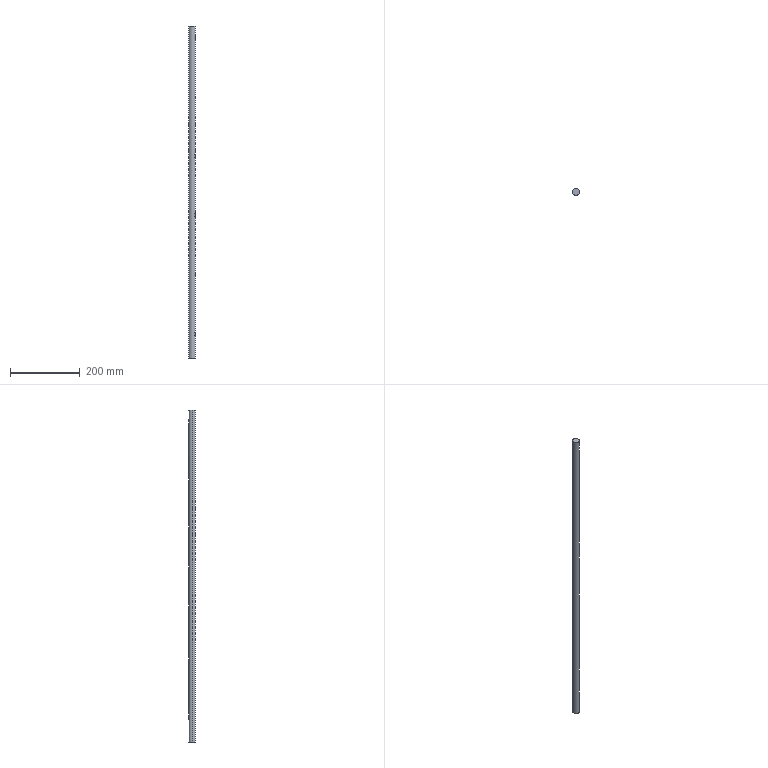Part | SolidWorks | features BaseBody 1 | 1 solid | 40 faces | box 20 x 20 x 952 mm | volume 298375 mm3 | plane 38 | cylinder 2 | commonest cylinder face diameters 20 x2
STEP:
#1=CARTESIAN_POINT('',(4.359,9.,914.5));
#2=VERTEX_POINT('',#1);
#3=CARTESIAN_POINT('',(-4.359,9.,914.5));
#4=VERTEX_POINT('',#3);
#5=CARTESIAN_POINT('',(0.,0.,914.5));
#6=DIRECTION('',(0.,0.,1.));
#7=DIRECTION('',(1.,0.,0.));
#8=AXIS2_PLACEMENT_3D('',#5,#6,#7);
#9=CIRCLE('',#8,10.);
#10=EDGE_CURVE('',#2,#4,#9,.T.);
#11=ORIENTED_EDGE('',*,*,#10,.F.);
#12=CARTESIAN_POINT('',(4.359,9.,924.5));
#13=VERTEX_POINT('',#12);
#14=CARTESIAN_POINT('',(4.359,9.,952.));
#15=DIRECTION('',(0.,0.,1.));
#16=VECTOR('',#15,1000.);
#17=LINE('',#14,#16);
#18=EDGE_CURVE('',#2,#13,#17,.T.);
#19=ORIENTED_EDGE('',*,*,#18,.T.);
#20=CARTESIAN_POINT('',(-4.359,9.,924.5));
#21=VERTEX_POINT('',#20);
#22=CARTESIAN_POINT('',(0.,0.,924.5));
#23=DIRECTION('',(0.,0.,1.));
#24=DIRECTION('',(1.,0.,0.));
#25=AXIS2_PLACEMENT_3D('',#22,#23,#24);
#26=CIRCLE('',#25,10.);
#27=EDGE_CURVE('',#13,#21,#26,.T.);
#28=ORIENTED_EDGE('',*,*,#27,.T.);
#29=CARTESIAN_POINT('',(-4.359,9.,952.));
#30=DIRECTION('',(0.,0.,-1.));
#31=VECTOR('',#30,1000.);
#32=LINE('',#29,#31);
#33=EDGE_CURVE('',#21,#4,#32,.T.);
#34=ORIENTED_EDGE('',*,*,#33,.T.);
#35=EDGE_LOOP('',(#11,#19,#28,#34));
#36=FACE_BOUND('',#35,.T.);
#37=CARTESIAN_POINT('',(4.359,9.,744.5));
#38=VERTEX_POINT('',#37);
#39=CARTESIAN_POINT('',(-4.359,9.,744.5));
#40=VERTEX_POINT('',#39);
#41=CARTESIAN_POINT('',(0.,0.,744.5));
#42=DIRECTION('',(0.,0.,1.));
#43=DIRECTION('',(1.,0.,0.));
#44=AXIS2_PLACEMENT_3D('',#41,#42,#43);
#45=CIRCLE('',#44,10.);
#46=EDGE_CURVE('',#38,#40,#45,.T.);
#47=ORIENTED_EDGE('',*,*,#46,.F.);
#48=CARTESIAN_POINT('',(4.359,9.,754.5));
#49=VERTEX_POINT('',#48);
#50=CARTESIAN_POINT('',(4.359,9.,952.));
#51=DIRECTION('',(0.,0.,1.));
#52=VECTOR('',#51,1000.);
#53=LINE('',#50,#52);
#54=EDGE_CURVE('',#38,#49,#53,.T.);
#55=ORIENTED_EDGE('',*,*,#54,.T.);
#56=CARTESIAN_POINT('',(-4.359,9.,754.5));
#57=VERTEX_POINT('',#56);
#58=CARTESIAN_POINT('',(0.,0.,754.5));
#59=DIRECTION('',(0.,0.,1.));
#60=DIRECTION('',(1.,0.,0.));
#61=AXIS2_PLACEMENT_3D('',#58,#59,#60);
#62=CIRCLE('',#61,10.);
#63=EDGE_CURVE('',#49,#57,#62,.T.);
#64=ORIENTED_EDGE('',*,*,#63,.T.);
#65=CARTESIAN_POINT('',(-4.359,9.,952.));
#66=DIRECTION('',(0.,0.,-1.));
#67=VECTOR('',#66,1000.);
#68=LINE('',#65,#67);
#69=EDGE_CURVE('',#57,#40,#68,.T.);
#70=ORIENTED_EDGE('',*,*,#69,.T.);
#71=EDGE_LOOP('',(#47,#55,#64,#70));
#72=FACE_BOUND('',#71,.T.);
#73=CARTESIAN_POINT('',(4.359,9.,574.5));
#74=VERTEX_POINT('',#73);
#75=CARTESIAN_POINT('',(-4.359,9.,574.5));
#76=VERTEX_POINT('',#75);
#77=CARTESIAN_POINT('',(0.,0.,574.5));
#78=DIRECTION('',(0.,0.,1.));
#79=DIRECTION('',(1.,0.,0.));
#80=AXIS2_PLACEMENT_3D('',#77,#78,#79);
#81=CIRCLE('',#80,10.);
#82=EDGE_CURVE('',#74,#76,#81,.T.);
#83=ORIENTED_EDGE('',*,*,#82,.F.);
#84=CARTESIAN_POINT('',(4.359,9.,584.5));
#85=VERTEX_POINT('',#84);
#86=CARTESIAN_POINT('',(4.359,9.,952.));
#87=DIRECTION('',(0.,0.,1.));
#88=VECTOR('',#87,1000.);
#89=LINE('',#86,#88);
#90=EDGE_CURVE('',#74,#85,#89,.T.);
#91=ORIENTED_EDGE('',*,*,#90,.T.);
#92=CARTESIAN_POINT('',(-4.359,9.,584.5));
#93=VERTEX_POINT('',#92);
#94=CARTESIAN_POINT('',(0.,0.,584.5));
#95=DIRECTION('',(0.,0.,1.));
#96=DIRECTION('',(1.,0.,0.));
#97=AXIS2_PLACEMENT_3D('',#94,#95,#96);
#98=CIRCLE('',#97,10.);
#99=EDGE_CURVE('',#85,#93,#98,.T.);
#100=ORIENTED_EDGE('',*,*,#99,.T.);
#101=CARTESIAN_POINT('',(-4.359,9.,952.));
#102=DIRECTION('',(0.,0.,-1.));
#103=VECTOR('',#102,1000.);
#104=LINE('',#101,#103);
#105=EDGE_CURVE('',#93,#76,#104,.T.);
#106=ORIENTED_EDGE('',*,*,#105,.T.);
#107=EDGE_LOOP('',(#83,#91,#100,#106));
#108=FACE_BOUND('',#107,.T.);
#109=CARTESIAN_POINT('',(4.359,9.,404.5));
#110=VERTEX_POINT('',#109);
#111=CARTESIAN_POINT('',(-4.359,9.,404.5));
#112=VERTEX_POINT('',#111);
#113=CARTESIAN_POINT('',(0.,0.,404.5));
#114=DIRECTION('',(0.,0.,1.));
#115=DIRECTION('',(1.,0.,0.));
#116=AXIS2_PLACEMENT_3D('',#113,#114,#115);
#117=CIRCLE('',#116,10.);
#118=EDGE_CURVE('',#110,#112,#117,.T.);
#119=ORIENTED_EDGE('',*,*,#118,.F.);
#120=CARTESIAN_POINT('',(4.359,9.,414.5));
#121=VERTEX_POINT('',#120);
#122=CARTESIAN_POINT('',(4.359,9.,952.));
#123=DIRECTION('',(0.,0.,1.));
#124=VECTOR('',#123,1000.);
#125=LINE('',#122,#124);
#126=EDGE_CURVE('',#110,#121,#125,.T.);
#127=ORIENTED_EDGE('',*,*,#126,.T.);
#128=CARTESIAN_POINT('',(-4.359,9.,414.5));
#129=VERTEX_POINT('',#128);
#130=CARTESIAN_POINT('',(0.,0.,414.5));
#131=DIRECTION('',(0.,0.,1.));
#132=DIRECTION('',(1.,0.,0.));
#133=AXIS2_PLACEMENT_3D('',#130,#131,#132);
#134=CIRCLE('',#133,10.);
#135=EDGE_CURVE('',#121,#129,#134,.T.);
#136=ORIENTED_EDGE('',*,*,#135,.T.);
#137=CARTESIAN_POINT('',(-4.359,9.,952.));
#138=DIRECTION('',(0.,0.,-1.));
#139=VECTOR('',#138,1000.);
#140=LINE('',#137,#139);
#141=EDGE_CURVE('',#129,#112,#140,.T.);
#142=ORIENTED_EDGE('',*,*,#141,.T.);
#143=EDGE_LOOP('',(#119,#127,#136,#142));
#144=FACE_BOUND('',#143,.T.);
#145=CARTESIAN_POINT('',(4.359,9.,234.5));
#146=VERTEX_POINT('',#145);
#147=CARTESIAN_POINT('',(-4.359,9.,234.5));
#148=VERTEX_POINT('',#147);
#149=CARTESIAN_POINT('',(0.,0.,234.5));
#150=DIRECTION('',(0.,0.,1.));
#151=DIRECTION('',(1.,0.,0.));
#152=AXIS2_PLACEMENT_3D('',#149,#150,#151);
#153=CIRCLE('',#152,10.);
#154=EDGE_CURVE('',#146,#148,#153,.T.);
#155=ORIENTED_EDGE('',*,*,#154,.F.);
#156=CARTESIAN_POINT('',(4.359,9.,244.5));
#157=VERTEX_POINT('',#156);
#158=CARTESIAN_POINT('',(4.359,9.,952.));
#159=DIRECTION('',(0.,0.,1.));
#160=VECTOR('',#159,1000.);
#161=LINE('',#158,#160);
#162=EDGE_CURVE('',#146,#157,#161,.T.);
#163=ORIENTED_EDGE('',*,*,#162,.T.);
#164=CARTESIAN_POINT('',(-4.359,9.,244.5));
#165=VERTEX_POINT('',#164);
#166=CARTESIAN_POINT('',(0.,0.,244.5));
#167=DIRECTION('',(0.,0.,1.));
#168=DIRECTION('',(1.,0.,0.));
#169=AXIS2_PLACEMENT_3D('',#166,#167,#168);
#170=CIRCLE('',#169,10.);
#171=EDGE_CURVE('',#157,#165,#170,.T.);
#172=ORIENTED_EDGE('',*,*,#171,.T.);
#173=CARTESIAN_POINT('',(-4.359,9.,952.));
#174=DIRECTION('',(0.,0.,-1.));
#175=VECTOR('',#174,1000.);
#176=LINE('',#173,#175);
#177=EDGE_CURVE('',#165,#148,#176,.T.);
#178=ORIENTED_EDGE('',*,*,#177,.T.);
#179=EDGE_LOOP('',(#155,#163,#172,#178));
#180=FACE_BOUND('',#179,.T.);
#181=CARTESIAN_POINT('',(4.359,9.,64.5));
#182=VERTEX_POINT('',#181);
#183=CARTESIAN_POINT('',(-4.359,9.,64.5));
#184=VERTEX_POINT('',#183);
#185=CARTESIAN_POINT('',(0.,0.,64.5));
#186=DIRECTION('',(0.,0.,1.));
#187=DIRECTION('',(1.,0.,0.));
#188=AXIS2_PLACEMENT_3D('',#185,#186,#187);
#189=CIRCLE('',#188,10.);
#190=EDGE_CURVE('',#182,#184,#189,.T.);
#191=ORIENTED_EDGE('',*,*,#190,.F.);
#192=CARTESIAN_POINT('',(4.359,9.,74.5));
#193=VERTEX_POINT('',#192);
#194=CARTESIAN_POINT('',(4.359,9.,952.));
#195=DIRECTION('',(0.,0.,1.));
#196=VECTOR('',#195,1000.);
#197=LINE('',#194,#196);
#198=EDGE_CURVE('',#182,#193,#197,.T.);
#199=ORIENTED_EDGE('',*,*,#198,.T.);
#200=CARTESIAN_POINT('',(-4.359,9.,74.5));
#201=VERTEX_POINT('',#200);
#202=CARTESIAN_POINT('',(0.,0.,74.5));
#203=DIRECTION('',(0.,0.,1.));
#204=DIRECTION('',(1.,0.,0.));
#205=AXIS2_PLACEMENT_3D('',#202,#203,#204);
#206=CIRCLE('',#205,10.);
#207=EDGE_CURVE('',#193,#201,#206,.T.);
#208=ORIENTED_EDGE('',*,*,#207,.T.);
#209=CARTESIAN_POINT('',(-4.359,9.,952.));
#210=DIRECTION('',(0.,0.,-1.));
#211=VECTOR('',#210,1000.);
#212=LINE('',#209,#211);
#213=EDGE_CURVE('',#201,#184,#212,.T.);
#214=ORIENTED_EDGE('',*,*,#213,.T.);
#215=EDGE_LOOP('',(#191,#199,#208,#214));
#216=FACE_BOUND('',#215,.T.);
#217=CARTESIAN_POINT('',(10.,0.,952.));
#218=VERTEX_POINT('',#217);
#219=CARTESIAN_POINT('',(-10.,0.,952.));
#220=VERTEX_POINT('',#219);
#221=CARTESIAN_POINT('',(0.,0.,952.));
#222=DIRECTION('',(0.,0.,1.));
#223=DIRECTION('',(1.,0.,0.));
#224=AXIS2_PLACEMENT_3D('',#221,#222,#223);
#225=CIRCLE('',#224,10.);
#226=EDGE_CURVE('',#218,#220,#225,.T.);
#227=ORIENTED_EDGE('',*,*,#226,.F.);
#228=CARTESIAN_POINT('',(10.,0.,0.));
#229=VERTEX_POINT('',#228);
#230=CARTESIAN_POINT('',(10.,0.,952.));
#231=DIRECTION('',(0.,0.,-1.));
#232=VECTOR('',#231,1000.);
#233=LINE('',#230,#232);
#234=EDGE_CURVE('',#218,#229,#233,.T.);
#235=ORIENTED_EDGE('',*,*,#234,.T.);
#236=CARTESIAN_POINT('',(-10.,0.,0.));
#237=VERTEX_POINT('',#236);
#238=CARTESIAN_POINT('',(0.,0.,0.));
#239=DIRECTION('',(0.,0.,1.));
#240=DIRECTION('',(1.,0.,0.));
#241=AXIS2_PLACEMENT_3D('',#238,#239,#240);
#242=CIRCLE('',#241,10.);
#243=EDGE_CURVE('',#229,#237,#242,.T.);
#244=ORIENTED_EDGE('',*,*,#243,.T.);
#245=CARTESIAN_POINT('',(-10.,0.,952.));
#246=DIRECTION('',(0.,0.,-1.));
#247=VECTOR('',#246,1000.);
#248=LINE('',#245,#247);
#249=EDGE_CURVE('',#220,#237,#248,.T.);
#250=ORIENTED_EDGE('',*,*,#249,.F.);
#251=EDGE_LOOP('',(#227,#235,#244,#250));
#252=FACE_OUTER_BOUND('',#251,.T.);
#253=CARTESIAN_POINT('',(0.,0.,952.));
#254=DIRECTION('',(0.,0.,-1.));
#255=DIRECTION('',(-1.,0.,0.));
#256=AXIS2_PLACEMENT_3D('',#253,#254,#255);
#257=CYLINDRICAL_SURFACE('',#256,10.);
#258=ADVANCED_FACE('',(#36,#72,#108,#144,#180,#216,#252),#257,.T.);
#259=CARTESIAN_POINT('',(9.974,-0.7251,74.5));
#260=VERTEX_POINT('',#259);
#261=CARTESIAN_POINT('',(5.615,-8.275,74.5));
#262=VERTEX_POINT('',#261);
#263=CARTESIAN_POINT('',(12.917,4.373,74.5));
#264=DIRECTION('',(-0.5,-0.866,0.));
#265=VECTOR('',#264,1000.);
#266=LINE('',#263,#265);
#267=EDGE_CURVE('',#260,#262,#266,.T.);
#268=ORIENTED_EDGE('',*,*,#267,.F.);
#269=CARTESIAN_POINT('',(0.,0.,74.5));
#270=DIRECTION('',(0.,0.,1.));
#271=DIRECTION('',(1.,0.,0.));
#272=AXIS2_PLACEMENT_3D('',#269,#270,#271);
#273=CIRCLE('',#272,10.);
#274=EDGE_CURVE('',#262,#260,#273,.T.);
#275=ORIENTED_EDGE('',*,*,#274,.F.);
#276=EDGE_LOOP('',(#268,#275));
#277=FACE_OUTER_BOUND('',#276,.T.);
#278=CARTESIAN_POINT('',(0.,0.,74.5));
#279=DIRECTION('',(0.,0.,1.));
#280=DIRECTION('',(1.,0.,0.));
#281=AXIS2_PLACEMENT_3D('',#278,#279,#280);
#282=PLANE('',#281);
#283=ADVANCED_FACE('',(#277),#282,.F.);
#284=CARTESIAN_POINT('',(5.615,-8.275,64.5));
#285=VERTEX_POINT('',#284);
#286=CARTESIAN_POINT('',(9.974,-0.7251,64.5));
#287=VERTEX_POINT('',#286);
#288=CARTESIAN_POINT('',(0.,0.,64.5));
#289=DIRECTION('',(0.,0.,1.));
#290=DIRECTION('',(1.,0.,0.));
#291=AXIS2_PLACEMENT_3D('',#288,#289,#290);
#292=CIRCLE('',#291,10.);
#293=EDGE_CURVE('',#285,#287,#292,.T.);
#294=ORIENTED_EDGE('',*,*,#293,.T.);
#295=CARTESIAN_POINT('',(12.917,4.373,64.5));
#296=DIRECTION('',(-0.5,-0.866,0.));
#297=VECTOR('',#296,1000.);
#298=LINE('',#295,#297);
#299=EDGE_CURVE('',#287,#285,#298,.T.);
#300=ORIENTED_EDGE('',*,*,#299,.T.);
#301=EDGE_LOOP('',(#294,#300));
#302=FACE_OUTER_BOUND('',#301,.T.);
#303=CARTESIAN_POINT('',(0.,0.,64.5));
#304=DIRECTION('',(0.,0.,1.));
#305=DIRECTION('',(1.,0.,0.));
#306=AXIS2_PLACEMENT_3D('',#303,#304,#305);
#307=PLANE('',#306);
#308=ADVANCED_FACE('',(#302),#307,.T.);
#309=ORIENTED_EDGE('',*,*,#267,.T.);
#310=CARTESIAN_POINT('',(5.615,-8.275,952.));
#311=DIRECTION('',(0.,0.,1.));
#312=VECTOR('',#311,1000.);
#313=LINE('',#310,#312);
#314=EDGE_CURVE('',#285,#262,#313,.T.);
#315=ORIENTED_EDGE('',*,*,#314,.F.);
#316=ORIENTED_EDGE('',*,*,#299,.F.);
#317=CARTESIAN_POINT('',(9.974,-0.7251,952.));
#318=DIRECTION('',(0.,0.,-1.));
#319=VECTOR('',#318,1000.);
#320=LINE('',#317,#319);
#321=EDGE_CURVE('',#260,#287,#320,.T.);
#322=ORIENTED_EDGE('',*,*,#321,.F.);
#323=EDGE_LOOP('',(#309,#315,#316,#322));
#324=FACE_OUTER_BOUND('',#323,.T.);
#325=CARTESIAN_POINT('',(12.917,4.373,64.5));
#326=DIRECTION('',(-0.866,0.5,0.));
#327=DIRECTION('',(0.,0.,1.));
#328=AXIS2_PLACEMENT_3D('',#325,#326,#327);
#329=PLANE('',#328);
#330=ADVANCED_FACE('',(#324),#329,.F.);
#331=CARTESIAN_POINT('',(-9.896,9.,74.5));
#332=DIRECTION('',(1.,0.,0.));
#333=VECTOR('',#332,1000.);
#334=LINE('',#331,#333);
#335=EDGE_CURVE('',#201,#193,#334,.T.);
#336=ORIENTED_EDGE('',*,*,#335,.F.);
#337=ORIENTED_EDGE('',*,*,#207,.F.);
#338=EDGE_LOOP('',(#336,#337));
#339=FACE_OUTER_BOUND('',#338,.T.);
#340=CARTESIAN_POINT('',(0.,0.,74.5));
#341=DIRECTION('',(0.,0.,1.));
#342=DIRECTION('',(1.,0.,0.));
#343=AXIS2_PLACEMENT_3D('',#340,#341,#342);
#344=PLANE('',#343);
#345=ADVANCED_FACE('',(#339),#344,.F.);
#346=ORIENTED_EDGE('',*,*,#190,.T.);
#347=CARTESIAN_POINT('',(-9.896,9.,64.5));
#348=DIRECTION('',(1.,0.,0.));
#349=VECTOR('',#348,1000.);
#350=LINE('',#347,#349);
#351=EDGE_CURVE('',#184,#182,#350,.T.);
#352=ORIENTED_EDGE('',*,*,#351,.T.);
#353=EDGE_LOOP('',(#346,#352));
#354=FACE_OUTER_BOUND('',#353,.T.);
#355=CARTESIAN_POINT('',(0.,0.,64.5));
#356=DIRECTION('',(0.,0.,1.));
#357=DIRECTION('',(1.,0.,0.));
#358=AXIS2_PLACEMENT_3D('',#355,#356,#357);
#359=PLANE('',#358);
#360=ADVANCED_FACE('',(#354),#359,.T.);
#361=ORIENTED_EDGE('',*,*,#335,.T.);
#362=ORIENTED_EDGE('',*,*,#198,.F.);
#363=ORIENTED_EDGE('',*,*,#351,.F.);
#364=ORIENTED_EDGE('',*,*,#213,.F.);
#365=EDGE_LOOP('',(#361,#362,#363,#364));
#366=FACE_OUTER_BOUND('',#365,.T.);
#367=CARTESIAN_POINT('',(-9.896,9.,64.5));
#368=DIRECTION('',(0.,-1.,0.));
#369=DIRECTION('',(0.,0.,-1.));
#370=AXIS2_PLACEMENT_3D('',#367,#368,#369);
#371=PLANE('',#370);
#372=ADVANCED_FACE('',(#366),#371,.F.);
#373=CARTESIAN_POINT('',(9.974,-0.7251,244.5));
#374=VERTEX_POINT('',#373);
#375=CARTESIAN_POINT('',(5.615,-8.275,244.5));
#376=VERTEX_POINT('',#375);
#377=CARTESIAN_POINT('',(12.917,4.373,244.5));
#378=DIRECTION('',(-0.5,-0.866,0.));
#379=VECTOR('',#378,1000.);
#380=LINE('',#377,#379);
#381=EDGE_CURVE('',#374,#376,#380,.T.);
#382=ORIENTED_EDGE('',*,*,#381,.F.);
#383=CARTESIAN_POINT('',(0.,0.,244.5));
#384=DIRECTION('',(0.,0.,1.));
#385=DIRECTION('',(1.,0.,0.));
#386=AXIS2_PLACEMENT_3D('',#383,#384,#385);
#387=CIRCLE('',#386,10.);
#388=EDGE_CURVE('',#376,#374,#387,.T.);
#389=ORIENTED_EDGE('',*,*,#388,.F.);
#390=EDGE_LOOP('',(#382,#389));
#391=FACE_OUTER_BOUND('',#390,.T.);
#392=CARTESIAN_POINT('',(0.,0.,244.5));
#393=DIRECTION('',(0.,0.,1.));
#394=DIRECTION('',(1.,0.,0.));
#395=AXIS2_PLACEMENT_3D('',#392,#393,#394);
#396=PLANE('',#395);
#397=ADVANCED_FACE('',(#391),#396,.F.);
#398=CARTESIAN_POINT('',(5.615,-8.275,234.5));
#399=VERTEX_POINT('',#398);
#400=CARTESIAN_POINT('',(9.974,-0.7251,234.5));
#401=VERTEX_POINT('',#400);
#402=CARTESIAN_POINT('',(0.,0.,234.5));
#403=DIRECTION('',(0.,0.,1.));
#404=DIRECTION('',(1.,0.,0.));
#405=AXIS2_PLACEMENT_3D('',#402,#403,#404);
#406=CIRCLE('',#405,10.);
#407=EDGE_CURVE('',#399,#401,#406,.T.);
#408=ORIENTED_EDGE('',*,*,#407,.T.);
#409=CARTESIAN_POINT('',(12.917,4.373,234.5));
#410=DIRECTION('',(-0.5,-0.866,0.));
#411=VECTOR('',#410,1000.);
#412=LINE('',#409,#411);
#413=EDGE_CURVE('',#401,#399,#412,.T.);
#414=ORIENTED_EDGE('',*,*,#413,.T.);
#415=EDGE_LOOP('',(#408,#414));
#416=FACE_OUTER_BOUND('',#415,.T.);
#417=CARTESIAN_POINT('',(0.,0.,234.5));
#418=DIRECTION('',(0.,0.,1.));
#419=DIRECTION('',(1.,0.,0.));
#420=AXIS2_PLACEMENT_3D('',#417,#418,#419);
#421=PLANE('',#420);
#422=ADVANCED_FACE('',(#416),#421,.T.);
#423=ORIENTED_EDGE('',*,*,#381,.T.);
#424=CARTESIAN_POINT('',(5.615,-8.275,952.));
#425=DIRECTION('',(0.,0.,1.));
#426=VECTOR('',#425,1000.);
#427=LINE('',#424,#426);
#428=EDGE_CURVE('',#399,#376,#427,.T.);
#429=ORIENTED_EDGE('',*,*,#428,.F.);
#430=ORIENTED_EDGE('',*,*,#413,.F.);
#431=CARTESIAN_POINT('',(9.974,-0.7251,952.));
#432=DIRECTION('',(0.,0.,-1.));
#433=VECTOR('',#432,1000.);
#434=LINE('',#431,#433);
#435=EDGE_CURVE('',#374,#401,#434,.T.);
#436=ORIENTED_EDGE('',*,*,#435,.F.);
#437=EDGE_LOOP('',(#423,#429,#430,#436));
#438=FACE_OUTER_BOUND('',#437,.T.);
#439=CARTESIAN_POINT('',(12.917,4.373,234.5));
#440=DIRECTION('',(-0.866,0.5,0.));
#441=DIRECTION('',(0.,0.,1.));
#442=AXIS2_PLACEMENT_3D('',#439,#440,#441);
#443=PLANE('',#442);
#444=ADVANCED_FACE('',(#438),#443,.F.);
#445=CARTESIAN_POINT('',(-9.896,9.,244.5));
#446=DIRECTION('',(1.,0.,0.));
#447=VECTOR('',#446,1000.);
#448=LINE('',#445,#447);
#449=EDGE_CURVE('',#165,#157,#448,.T.);
#450=ORIENTED_EDGE('',*,*,#449,.F.);
#451=ORIENTED_EDGE('',*,*,#171,.F.);
#452=EDGE_LOOP('',(#450,#451));
#453=FACE_OUTER_BOUND('',#452,.T.);
#454=CARTESIAN_POINT('',(0.,0.,244.5));
#455=DIRECTION('',(0.,0.,1.));
#456=DIRECTION('',(1.,0.,0.));
#457=AXIS2_PLACEMENT_3D('',#454,#455,#456);
#458=PLANE('',#457);
#459=ADVANCED_FACE('',(#453),#458,.F.);
#460=ORIENTED_EDGE('',*,*,#154,.T.);
#461=CARTESIAN_POINT('',(-9.896,9.,234.5));
#462=DIRECTION('',(1.,0.,0.));
#463=VECTOR('',#462,1000.);
#464=LINE('',#461,#463);
#465=EDGE_CURVE('',#148,#146,#464,.T.);
#466=ORIENTED_EDGE('',*,*,#465,.T.);
#467=EDGE_LOOP('',(#460,#466));
#468=FACE_OUTER_BOUND('',#467,.T.);
#469=CARTESIAN_POINT('',(0.,0.,234.5));
#470=DIRECTION('',(0.,0.,1.));
#471=DIRECTION('',(1.,0.,0.));
#472=AXIS2_PLACEMENT_3D('',#469,#470,#471);
#473=PLANE('',#472);
#474=ADVANCED_FACE('',(#468),#473,.T.);
#475=ORIENTED_EDGE('',*,*,#449,.T.);
#476=ORIENTED_EDGE('',*,*,#162,.F.);
#477=ORIENTED_EDGE('',*,*,#465,.F.);
#478=ORIENTED_EDGE('',*,*,#177,.F.);
#479=EDGE_LOOP('',(#475,#476,#477,#478));
#480=FACE_OUTER_BOUND('',#479,.T.);
#481=CARTESIAN_POINT('',(-9.896,9.,234.5));
#482=DIRECTION('',(0.,-1.,0.));
#483=DIRECTION('',(0.,0.,-1.));
#484=AXIS2_PLACEMENT_3D('',#481,#482,#483);
#485=PLANE('',#484);
#486=ADVANCED_FACE('',(#480),#485,.F.);
#487=CARTESIAN_POINT('',(9.974,-0.7251,414.5));
#488=VERTEX_POINT('',#487);
#489=CARTESIAN_POINT('',(5.615,-8.275,414.5));
#490=VERTEX_POINT('',#489);
#491=CARTESIAN_POINT('',(12.917,4.373,414.5));
#492=DIRECTION('',(-0.5,-0.866,0.));
#493=VECTOR('',#492,1000.);
#494=LINE('',#491,#493);
#495=EDGE_CURVE('',#488,#490,#494,.T.);
#496=ORIENTED_EDGE('',*,*,#495,.F.);
#497=CARTESIAN_POINT('',(0.,0.,414.5));
#498=DIRECTION('',(0.,0.,1.));
#499=DIRECTION('',(1.,0.,0.));
#500=AXIS2_PLACEMENT_3D('',#497,#498,#499);
#501=CIRCLE('',#500,10.);
#502=EDGE_CURVE('',#490,#488,#501,.T.);
#503=ORIENTED_EDGE('',*,*,#502,.F.);
#504=EDGE_LOOP('',(#496,#503));
#505=FACE_OUTER_BOUND('',#504,.T.);
#506=CARTESIAN_POINT('',(0.,0.,414.5));
#507=DIRECTION('',(0.,0.,1.));
#508=DIRECTION('',(1.,0.,0.));
#509=AXIS2_PLACEMENT_3D('',#506,#507,#508);
#510=PLANE('',#509);
#511=ADVANCED_FACE('',(#505),#510,.F.);
#512=CARTESIAN_POINT('',(5.615,-8.275,404.5));
#513=VERTEX_POINT('',#512);
#514=CARTESIAN_POINT('',(9.974,-0.7251,404.5));
#515=VERTEX_POINT('',#514);
#516=CARTESIAN_POINT('',(0.,0.,404.5));
#517=DIRECTION('',(0.,0.,1.));
#518=DIRECTION('',(1.,0.,0.));
#519=AXIS2_PLACEMENT_3D('',#516,#517,#518);
#520=CIRCLE('',#519,10.);
#521=EDGE_CURVE('',#513,#515,#520,.T.);
#522=ORIENTED_EDGE('',*,*,#521,.T.);
#523=CARTESIAN_POINT('',(12.917,4.373,404.5));
#524=DIRECTION('',(-0.5,-0.866,0.));
#525=VECTOR('',#524,1000.);
#526=LINE('',#523,#525);
#527=EDGE_CURVE('',#515,#513,#526,.T.);
#528=ORIENTED_EDGE('',*,*,#527,.T.);
#529=EDGE_LOOP('',(#522,#528));
#530=FACE_OUTER_BOUND('',#529,.T.);
#531=CARTESIAN_POINT('',(0.,0.,404.5));
#532=DIRECTION('',(0.,0.,1.));
#533=DIRECTION('',(1.,0.,0.));
#534=AXIS2_PLACEMENT_3D('',#531,#532,#533);
#535=PLANE('',#534);
#536=ADVANCED_FACE('',(#530),#535,.T.);
#537=ORIENTED_EDGE('',*,*,#495,.T.);
#538=CARTESIAN_POINT('',(5.615,-8.275,952.));
#539=DIRECTION('',(0.,0.,1.));
#540=VECTOR('',#539,1000.);
#541=LINE('',#538,#540);
#542=EDGE_CURVE('',#513,#490,#541,.T.);
#543=ORIENTED_EDGE('',*,*,#542,.F.);
#544=ORIENTED_EDGE('',*,*,#527,.F.);
#545=CARTESIAN_POINT('',(9.974,-0.7251,952.));
#546=DIRECTION('',(0.,0.,-1.));
#547=VECTOR('',#546,1000.);
#548=LINE('',#545,#547);
#549=EDGE_CURVE('',#488,#515,#548,.T.);
#550=ORIENTED_EDGE('',*,*,#549,.F.);
#551=EDGE_LOOP('',(#537,#543,#544,#550));
#552=FACE_OUTER_BOUND('',#551,.T.);
#553=CARTESIAN_POINT('',(12.917,4.373,404.5));
#554=DIRECTION('',(-0.866,0.5,0.));
#555=DIRECTION('',(0.,0.,1.));
#556=AXIS2_PLACEMENT_3D('',#553,#554,#555);
#557=PLANE('',#556);
#558=ADVANCED_FACE('',(#552),#557,.F.);
#559=CARTESIAN_POINT('',(-9.896,9.,414.5));
#560=DIRECTION('',(1.,0.,0.));
#561=VECTOR('',#560,1000.);
#562=LINE('',#559,#561);
#563=EDGE_CURVE('',#129,#121,#562,.T.);
#564=ORIENTED_EDGE('',*,*,#563,.F.);
#565=ORIENTED_EDGE('',*,*,#135,.F.);
#566=EDGE_LOOP('',(#564,#565));
#567=FACE_OUTER_BOUND('',#566,.T.);
#568=CARTESIAN_POINT('',(0.,0.,414.5));
#569=DIRECTION('',(0.,0.,1.));
#570=DIRECTION('',(1.,0.,0.));
#571=AXIS2_PLACEMENT_3D('',#568,#569,#570);
#572=PLANE('',#571);
#573=ADVANCED_FACE('',(#567),#572,.F.);
#574=ORIENTED_EDGE('',*,*,#118,.T.);
#575=CARTESIAN_POINT('',(-9.896,9.,404.5));
#576=DIRECTION('',(1.,0.,0.));
#577=VECTOR('',#576,1000.);
#578=LINE('',#575,#577);
#579=EDGE_CURVE('',#112,#110,#578,.T.);
#580=ORIENTED_EDGE('',*,*,#579,.T.);
#581=EDGE_LOOP('',(#574,#580));
#582=FACE_OUTER_BOUND('',#581,.T.);
#583=CARTESIAN_POINT('',(0.,0.,404.5));
#584=DIRECTION('',(0.,0.,1.));
#585=DIRECTION('',(1.,0.,0.));
#586=AXIS2_PLACEMENT_3D('',#583,#584,#585);
#587=PLANE('',#586);
#588=ADVANCED_FACE('',(#582),#587,.T.);
#589=ORIENTED_EDGE('',*,*,#563,.T.);
#590=ORIENTED_EDGE('',*,*,#126,.F.);
#591=ORIENTED_EDGE('',*,*,#579,.F.);
#592=ORIENTED_EDGE('',*,*,#141,.F.);
#593=EDGE_LOOP('',(#589,#590,#591,#592));
#594=FACE_OUTER_BOUND('',#593,.T.);
#595=CARTESIAN_POINT('',(-9.896,9.,404.5));
#596=DIRECTION('',(0.,-1.,0.));
#597=DIRECTION('',(0.,0.,-1.));
#598=AXIS2_PLACEMENT_3D('',#595,#596,#597);
#599=PLANE('',#598);
#600=ADVANCED_FACE('',(#594),#599,.F.);
#601=CARTESIAN_POINT('',(9.974,-0.7251,584.5));
#602=VERTEX_POINT('',#601);
#603=CARTESIAN_POINT('',(5.615,-8.275,584.5));
#604=VERTEX_POINT('',#603);
#605=CARTESIAN_POINT('',(12.917,4.373,584.5));
#606=DIRECTION('',(-0.5,-0.866,0.));
#607=VECTOR('',#606,1000.);
#608=LINE('',#605,#607);
#609=EDGE_CURVE('',#602,#604,#608,.T.);
#610=ORIENTED_EDGE('',*,*,#609,.F.);
#611=CARTESIAN_POINT('',(0.,0.,584.5));
#612=DIRECTION('',(0.,0.,1.));
#613=DIRECTION('',(1.,0.,0.));
#614=AXIS2_PLACEMENT_3D('',#611,#612,#613);
#615=CIRCLE('',#614,10.);
#616=EDGE_CURVE('',#604,#602,#615,.T.);
#617=ORIENTED_EDGE('',*,*,#616,.F.);
#618=EDGE_LOOP('',(#610,#617));
#619=FACE_OUTER_BOUND('',#618,.T.);
#620=CARTESIAN_POINT('',(0.,0.,584.5));
#621=DIRECTION('',(0.,0.,1.));
#622=DIRECTION('',(1.,0.,0.));
#623=AXIS2_PLACEMENT_3D('',#620,#621,#622);
#624=PLANE('',#623);
#625=ADVANCED_FACE('',(#619),#624,.F.);
#626=CARTESIAN_POINT('',(5.615,-8.275,574.5));
#627=VERTEX_POINT('',#626);
#628=CARTESIAN_POINT('',(9.974,-0.7251,574.5));
#629=VERTEX_POINT('',#628);
#630=CARTESIAN_POINT('',(0.,0.,574.5));
#631=DIRECTION('',(0.,0.,1.));
#632=DIRECTION('',(1.,0.,0.));
#633=AXIS2_PLACEMENT_3D('',#630,#631,#632);
#634=CIRCLE('',#633,10.);
#635=EDGE_CURVE('',#627,#629,#634,.T.);
#636=ORIENTED_EDGE('',*,*,#635,.T.);
#637=CARTESIAN_POINT('',(12.917,4.373,574.5));
#638=DIRECTION('',(-0.5,-0.866,0.));
#639=VECTOR('',#638,1000.);
#640=LINE('',#637,#639);
#641=EDGE_CURVE('',#629,#627,#640,.T.);
#642=ORIENTED_EDGE('',*,*,#641,.T.);
#643=EDGE_LOOP('',(#636,#642));
#644=FACE_OUTER_BOUND('',#643,.T.);
#645=CARTESIAN_POINT('',(0.,0.,574.5));
#646=DIRECTION('',(0.,0.,1.));
#647=DIRECTION('',(1.,0.,0.));
#648=AXIS2_PLACEMENT_3D('',#645,#646,#647);
#649=PLANE('',#648);
#650=ADVANCED_FACE('',(#644),#649,.T.);
#651=ORIENTED_EDGE('',*,*,#609,.T.);
#652=CARTESIAN_POINT('',(5.615,-8.275,952.));
#653=DIRECTION('',(0.,0.,1.));
#654=VECTOR('',#653,1000.);
#655=LINE('',#652,#654);
#656=EDGE_CURVE('',#627,#604,#655,.T.);
#657=ORIENTED_EDGE('',*,*,#656,.F.);
#658=ORIENTED_EDGE('',*,*,#641,.F.);
#659=CARTESIAN_POINT('',(9.974,-0.7251,952.));
#660=DIRECTION('',(0.,0.,-1.));
#661=VECTOR('',#660,1000.);
#662=LINE('',#659,#661);
#663=EDGE_CURVE('',#602,#629,#662,.T.);
#664=ORIENTED_EDGE('',*,*,#663,.F.);
#665=EDGE_LOOP('',(#651,#657,#658,#664));
#666=FACE_OUTER_BOUND('',#665,.T.);
#667=CARTESIAN_POINT('',(12.917,4.373,574.5));
#668=DIRECTION('',(-0.866,0.5,0.));
#669=DIRECTION('',(0.,0.,1.));
#670=AXIS2_PLACEMENT_3D('',#667,#668,#669);
#671=PLANE('',#670);
#672=ADVANCED_FACE('',(#666),#671,.F.);
#673=CARTESIAN_POINT('',(-9.896,9.,584.5));
#674=DIRECTION('',(1.,0.,0.));
#675=VECTOR('',#674,1000.);
#676=LINE('',#673,#675);
#677=EDGE_CURVE('',#93,#85,#676,.T.);
#678=ORIENTED_EDGE('',*,*,#677,.F.);
#679=ORIENTED_EDGE('',*,*,#99,.F.);
#680=EDGE_LOOP('',(#678,#679));
#681=FACE_OUTER_BOUND('',#680,.T.);
#682=CARTESIAN_POINT('',(0.,0.,584.5));
#683=DIRECTION('',(0.,0.,1.));
#684=DIRECTION('',(1.,0.,0.));
#685=AXIS2_PLACEMENT_3D('',#682,#683,#684);
#686=PLANE('',#685);
#687=ADVANCED_FACE('',(#681),#686,.F.);
#688=ORIENTED_EDGE('',*,*,#82,.T.);
#689=CARTESIAN_POINT('',(-9.896,9.,574.5));
#690=DIRECTION('',(1.,0.,0.));
#691=VECTOR('',#690,1000.);
#692=LINE('',#689,#691);
#693=EDGE_CURVE('',#76,#74,#692,.T.);
#694=ORIENTED_EDGE('',*,*,#693,.T.);
#695=EDGE_LOOP('',(#688,#694));
#696=FACE_OUTER_BOUND('',#695,.T.);
#697=CARTESIAN_POINT('',(0.,0.,574.5));
#698=DIRECTION('',(0.,0.,1.));
#699=DIRECTION('',(1.,0.,0.));
#700=AXIS2_PLACEMENT_3D('',#697,#698,#699);
#701=PLANE('',#700);
#702=ADVANCED_FACE('',(#696),#701,.T.);
#703=ORIENTED_EDGE('',*,*,#677,.T.);
#704=ORIENTED_EDGE('',*,*,#90,.F.);
#705=ORIENTED_EDGE('',*,*,#693,.F.);
#706=ORIENTED_EDGE('',*,*,#105,.F.);
#707=EDGE_LOOP('',(#703,#704,#705,#706));
#708=FACE_OUTER_BOUND('',#707,.T.);
#709=CARTESIAN_POINT('',(-9.896,9.,574.5));
#710=DIRECTION('',(0.,-1.,0.));
#711=DIRECTION('',(0.,0.,-1.));
#712=AXIS2_PLACEMENT_3D('',#709,#710,#711);
#713=PLANE('',#712);
#714=ADVANCED_FACE('',(#708),#713,.F.);
#715=CARTESIAN_POINT('',(9.974,-0.7251,754.5));
#716=VERTEX_POINT('',#715);
#717=CARTESIAN_POINT('',(5.615,-8.275,754.5));
#718=VERTEX_POINT('',#717);
#719=CARTESIAN_POINT('',(12.917,4.373,754.5));
#720=DIRECTION('',(-0.5,-0.866,0.));
#721=VECTOR('',#720,1000.);
#722=LINE('',#719,#721);
#723=EDGE_CURVE('',#716,#718,#722,.T.);
#724=ORIENTED_EDGE('',*,*,#723,.F.);
#725=CARTESIAN_POINT('',(0.,0.,754.5));
#726=DIRECTION('',(0.,0.,1.));
#727=DIRECTION('',(1.,0.,0.));
#728=AXIS2_PLACEMENT_3D('',#725,#726,#727);
#729=CIRCLE('',#728,10.);
#730=EDGE_CURVE('',#718,#716,#729,.T.);
#731=ORIENTED_EDGE('',*,*,#730,.F.);
#732=EDGE_LOOP('',(#724,#731));
#733=FACE_OUTER_BOUND('',#732,.T.);
#734=CARTESIAN_POINT('',(0.,0.,754.5));
#735=DIRECTION('',(0.,0.,1.));
#736=DIRECTION('',(1.,0.,0.));
#737=AXIS2_PLACEMENT_3D('',#734,#735,#736);
#738=PLANE('',#737);
#739=ADVANCED_FACE('',(#733),#738,.F.);
#740=CARTESIAN_POINT('',(5.615,-8.275,744.5));
#741=VERTEX_POINT('',#740);
#742=CARTESIAN_POINT('',(9.974,-0.7251,744.5));
#743=VERTEX_POINT('',#742);
#744=CARTESIAN_POINT('',(0.,0.,744.5));
#745=DIRECTION('',(0.,0.,1.));
#746=DIRECTION('',(1.,0.,0.));
#747=AXIS2_PLACEMENT_3D('',#744,#745,#746);
#748=CIRCLE('',#747,10.);
#749=EDGE_CURVE('',#741,#743,#748,.T.);
#750=ORIENTED_EDGE('',*,*,#749,.T.);
#751=CARTESIAN_POINT('',(12.917,4.373,744.5));
#752=DIRECTION('',(-0.5,-0.866,0.));
#753=VECTOR('',#752,1000.);
#754=LINE('',#751,#753);
#755=EDGE_CURVE('',#743,#741,#754,.T.);
#756=ORIENTED_EDGE('',*,*,#755,.T.);
#757=EDGE_LOOP('',(#750,#756));
#758=FACE_OUTER_BOUND('',#757,.T.);
#759=CARTESIAN_POINT('',(0.,0.,744.5));
#760=DIRECTION('',(0.,0.,1.));
#761=DIRECTION('',(1.,0.,0.));
#762=AXIS2_PLACEMENT_3D('',#759,#760,#761);
#763=PLANE('',#762);
#764=ADVANCED_FACE('',(#758),#763,.T.);
#765=ORIENTED_EDGE('',*,*,#723,.T.);
#766=CARTESIAN_POINT('',(5.615,-8.275,952.));
#767=DIRECTION('',(0.,0.,1.));
#768=VECTOR('',#767,1000.);
#769=LINE('',#766,#768);
#770=EDGE_CURVE('',#741,#718,#769,.T.);
#771=ORIENTED_EDGE('',*,*,#770,.F.);
#772=ORIENTED_EDGE('',*,*,#755,.F.);
#773=CARTESIAN_POINT('',(9.974,-0.7251,952.));
#774=DIRECTION('',(0.,0.,-1.));
#775=VECTOR('',#774,1000.);
#776=LINE('',#773,#775);
#777=EDGE_CURVE('',#716,#743,#776,.T.);
#778=ORIENTED_EDGE('',*,*,#777,.F.);
#779=EDGE_LOOP('',(#765,#771,#772,#778));
#780=FACE_OUTER_BOUND('',#779,.T.);
#781=CARTESIAN_POINT('',(12.917,4.373,744.5));
#782=DIRECTION('',(-0.866,0.5,0.));
#783=DIRECTION('',(0.,0.,1.));
#784=AXIS2_PLACEMENT_3D('',#781,#782,#783);
#785=PLANE('',#784);
#786=ADVANCED_FACE('',(#780),#785,.F.);
#787=CARTESIAN_POINT('',(-9.896,9.,754.5));
#788=DIRECTION('',(1.,0.,0.));
#789=VECTOR('',#788,1000.);
#790=LINE('',#787,#789);
#791=EDGE_CURVE('',#57,#49,#790,.T.);
#792=ORIENTED_EDGE('',*,*,#791,.F.);
#793=ORIENTED_EDGE('',*,*,#63,.F.);
#794=EDGE_LOOP('',(#792,#793));
#795=FACE_OUTER_BOUND('',#794,.T.);
#796=CARTESIAN_POINT('',(0.,0.,754.5));
#797=DIRECTION('',(0.,0.,1.));
#798=DIRECTION('',(1.,0.,0.));
#799=AXIS2_PLACEMENT_3D('',#796,#797,#798);
#800=PLANE('',#799);
#801=ADVANCED_FACE('',(#795),#800,.F.);
#802=ORIENTED_EDGE('',*,*,#46,.T.);
#803=CARTESIAN_POINT('',(-9.896,9.,744.5));
#804=DIRECTION('',(1.,0.,0.));
#805=VECTOR('',#804,1000.);
#806=LINE('',#803,#805);
#807=EDGE_CURVE('',#40,#38,#806,.T.);
#808=ORIENTED_EDGE('',*,*,#807,.T.);
#809=EDGE_LOOP('',(#802,#808));
#810=FACE_OUTER_BOUND('',#809,.T.);
#811=CARTESIAN_POINT('',(0.,0.,744.5));
#812=DIRECTION('',(0.,0.,1.));
#813=DIRECTION('',(1.,0.,0.));
#814=AXIS2_PLACEMENT_3D('',#811,#812,#813);
#815=PLANE('',#814);
#816=ADVANCED_FACE('',(#810),#815,.T.);
#817=ORIENTED_EDGE('',*,*,#791,.T.);
#818=ORIENTED_EDGE('',*,*,#54,.F.);
#819=ORIENTED_EDGE('',*,*,#807,.F.);
#820=ORIENTED_EDGE('',*,*,#69,.F.);
#821=EDGE_LOOP('',(#817,#818,#819,#820));
#822=FACE_OUTER_BOUND('',#821,.T.);
#823=CARTESIAN_POINT('',(-9.896,9.,744.5));
#824=DIRECTION('',(0.,-1.,0.));
#825=DIRECTION('',(0.,0.,-1.));
#826=AXIS2_PLACEMENT_3D('',#823,#824,#825);
#827=PLANE('',#826);
#828=ADVANCED_FACE('',(#822),#827,.F.);
#829=CARTESIAN_POINT('',(9.974,-0.7251,924.5));
#830=VERTEX_POINT('',#829);
#831=CARTESIAN_POINT('',(5.615,-8.275,924.5));
#832=VERTEX_POINT('',#831);
#833=CARTESIAN_POINT('',(12.917,4.373,924.5));
#834=DIRECTION('',(-0.5,-0.866,0.));
#835=VECTOR('',#834,1000.);
#836=LINE('',#833,#835);
#837=EDGE_CURVE('',#830,#832,#836,.T.);
#838=ORIENTED_EDGE('',*,*,#837,.F.);
#839=CARTESIAN_POINT('',(0.,0.,924.5));
#840=DIRECTION('',(0.,0.,1.));
#841=DIRECTION('',(1.,0.,0.));
#842=AXIS2_PLACEMENT_3D('',#839,#840,#841);
#843=CIRCLE('',#842,10.);
#844=EDGE_CURVE('',#832,#830,#843,.T.);
#845=ORIENTED_EDGE('',*,*,#844,.F.);
#846=EDGE_LOOP('',(#838,#845));
#847=FACE_OUTER_BOUND('',#846,.T.);
#848=CARTESIAN_POINT('',(0.,0.,924.5));
#849=DIRECTION('',(0.,0.,1.));
#850=DIRECTION('',(1.,0.,0.));
#851=AXIS2_PLACEMENT_3D('',#848,#849,#850);
#852=PLANE('',#851);
#853=ADVANCED_FACE('',(#847),#852,.F.);
#854=CARTESIAN_POINT('',(5.615,-8.275,914.5));
#855=VERTEX_POINT('',#854);
#856=CARTESIAN_POINT('',(9.974,-0.7251,914.5));
#857=VERTEX_POINT('',#856);
#858=CARTESIAN_POINT('',(0.,0.,914.5));
#859=DIRECTION('',(0.,0.,1.));
#860=DIRECTION('',(1.,0.,0.));
#861=AXIS2_PLACEMENT_3D('',#858,#859,#860);
#862=CIRCLE('',#861,10.);
#863=EDGE_CURVE('',#855,#857,#862,.T.);
#864=ORIENTED_EDGE('',*,*,#863,.T.);
#865=CARTESIAN_POINT('',(12.917,4.373,914.5));
#866=DIRECTION('',(-0.5,-0.866,0.));
#867=VECTOR('',#866,1000.);
#868=LINE('',#865,#867);
#869=EDGE_CURVE('',#857,#855,#868,.T.);
#870=ORIENTED_EDGE('',*,*,#869,.T.);
#871=EDGE_LOOP('',(#864,#870));
#872=FACE_OUTER_BOUND('',#871,.T.);
#873=CARTESIAN_POINT('',(0.,0.,914.5));
#874=DIRECTION('',(0.,0.,1.));
#875=DIRECTION('',(1.,0.,0.));
#876=AXIS2_PLACEMENT_3D('',#873,#874,#875);
#877=PLANE('',#876);
#878=ADVANCED_FACE('',(#872),#877,.T.);
#879=ORIENTED_EDGE('',*,*,#837,.T.);
#880=CARTESIAN_POINT('',(5.615,-8.275,952.));
#881=DIRECTION('',(0.,0.,1.));
#882=VECTOR('',#881,1000.);
#883=LINE('',#880,#882);
#884=EDGE_CURVE('',#855,#832,#883,.T.);
#885=ORIENTED_EDGE('',*,*,#884,.F.);
#886=ORIENTED_EDGE('',*,*,#869,.F.);
#887=CARTESIAN_POINT('',(9.974,-0.7251,952.));
#888=DIRECTION('',(0.,0.,-1.));
#889=VECTOR('',#888,1000.);
#890=LINE('',#887,#889);
#891=EDGE_CURVE('',#830,#857,#890,.T.);
#892=ORIENTED_EDGE('',*,*,#891,.F.);
#893=EDGE_LOOP('',(#879,#885,#886,#892));
#894=FACE_OUTER_BOUND('',#893,.T.);
#895=CARTESIAN_POINT('',(12.917,4.373,914.5));
#896=DIRECTION('',(-0.866,0.5,0.));
#897=DIRECTION('',(0.,0.,1.));
#898=AXIS2_PLACEMENT_3D('',#895,#896,#897);
#899=PLANE('',#898);
#900=ADVANCED_FACE('',(#894),#899,.F.);
#901=CARTESIAN_POINT('',(-9.896,9.,924.5));
#902=DIRECTION('',(1.,0.,0.));
#903=VECTOR('',#902,1000.);
#904=LINE('',#901,#903);
#905=EDGE_CURVE('',#21,#13,#904,.T.);
#906=ORIENTED_EDGE('',*,*,#905,.F.);
#907=ORIENTED_EDGE('',*,*,#27,.F.);
#908=EDGE_LOOP('',(#906,#907));
#909=FACE_OUTER_BOUND('',#908,.T.);
#910=CARTESIAN_POINT('',(0.,0.,924.5));
#911=DIRECTION('',(0.,0.,1.));
#912=DIRECTION('',(1.,0.,0.));
#913=AXIS2_PLACEMENT_3D('',#910,#911,#912);
#914=PLANE('',#913);
#915=ADVANCED_FACE('',(#909),#914,.F.);
#916=ORIENTED_EDGE('',*,*,#10,.T.);
#917=CARTESIAN_POINT('',(-9.896,9.,914.5));
#918=DIRECTION('',(1.,0.,0.));
#919=VECTOR('',#918,1000.);
#920=LINE('',#917,#919);
#921=EDGE_CURVE('',#4,#2,#920,.T.);
#922=ORIENTED_EDGE('',*,*,#921,.T.);
#923=EDGE_LOOP('',(#916,#922));
#924=FACE_OUTER_BOUND('',#923,.T.);
#925=CARTESIAN_POINT('',(0.,0.,914.5));
#926=DIRECTION('',(0.,0.,1.));
#927=DIRECTION('',(1.,0.,0.));
#928=AXIS2_PLACEMENT_3D('',#925,#926,#927);
#929=PLANE('',#928);
#930=ADVANCED_FACE('',(#924),#929,.T.);
#931=ORIENTED_EDGE('',*,*,#905,.T.);
#932=ORIENTED_EDGE('',*,*,#18,.F.);
#933=ORIENTED_EDGE('',*,*,#921,.F.);
#934=ORIENTED_EDGE('',*,*,#33,.F.);
#935=EDGE_LOOP('',(#931,#932,#933,#934));
#936=FACE_OUTER_BOUND('',#935,.T.);
#937=CARTESIAN_POINT('',(-9.896,9.,914.5));
#938=DIRECTION('',(0.,-1.,0.));
#939=DIRECTION('',(0.,0.,-1.));
#940=AXIS2_PLACEMENT_3D('',#937,#938,#939);
#941=PLANE('',#940);
#942=ADVANCED_FACE('',(#936),#941,.F.);
#943=CARTESIAN_POINT('',(0.,0.,0.));
#944=DIRECTION('',(0.,0.,1.));
#945=DIRECTION('',(1.,0.,0.));
#946=AXIS2_PLACEMENT_3D('',#943,#944,#945);
#947=CIRCLE('',#946,10.);
#948=EDGE_CURVE('',#237,#229,#947,.T.);
#949=ORIENTED_EDGE('',*,*,#948,.F.);
#950=ORIENTED_EDGE('',*,*,#243,.F.);
#951=EDGE_LOOP('',(#949,#950));
#952=FACE_OUTER_BOUND('',#951,.T.);
#953=CARTESIAN_POINT('',(0.,0.,0.));
#954=DIRECTION('',(0.,0.,1.));
#955=DIRECTION('',(1.,0.,0.));
#956=AXIS2_PLACEMENT_3D('',#953,#954,#955);
#957=PLANE('',#956);
#958=ADVANCED_FACE('',(#952),#957,.F.);
#959=CARTESIAN_POINT('',(0.,0.,952.));
#960=DIRECTION('',(0.,0.,1.));
#961=DIRECTION('',(1.,0.,0.));
#962=AXIS2_PLACEMENT_3D('',#959,#960,#961);
#963=CIRCLE('',#962,10.);
#964=EDGE_CURVE('',#220,#218,#963,.T.);
#965=ORIENTED_EDGE('',*,*,#964,.T.);
#966=ORIENTED_EDGE('',*,*,#226,.T.);
#967=EDGE_LOOP('',(#965,#966));
#968=FACE_OUTER_BOUND('',#967,.T.);
#969=CARTESIAN_POINT('',(0.,0.,952.));
#970=DIRECTION('',(0.,0.,1.));
#971=DIRECTION('',(1.,0.,0.));
#972=AXIS2_PLACEMENT_3D('',#969,#970,#971);
#973=PLANE('',#972);
#974=ADVANCED_FACE('',(#968),#973,.T.);
#975=ORIENTED_EDGE('',*,*,#234,.F.);
#976=ORIENTED_EDGE('',*,*,#964,.F.);
#977=ORIENTED_EDGE('',*,*,#249,.T.);
#978=ORIENTED_EDGE('',*,*,#948,.T.);
#979=EDGE_LOOP('',(#975,#976,#977,#978));
#980=FACE_OUTER_BOUND('',#979,.T.);
#981=ORIENTED_EDGE('',*,*,#293,.F.);
#982=ORIENTED_EDGE('',*,*,#314,.T.);
#983=ORIENTED_EDGE('',*,*,#274,.T.);
#984=ORIENTED_EDGE('',*,*,#321,.T.);
#985=EDGE_LOOP('',(#981,#982,#983,#984));
#986=FACE_BOUND('',#985,.T.);
#987=ORIENTED_EDGE('',*,*,#407,.F.);
#988=ORIENTED_EDGE('',*,*,#428,.T.);
#989=ORIENTED_EDGE('',*,*,#388,.T.);
#990=ORIENTED_EDGE('',*,*,#435,.T.);
#991=EDGE_LOOP('',(#987,#988,#989,#990));
#992=FACE_BOUND('',#991,.T.);
#993=ORIENTED_EDGE('',*,*,#521,.F.);
#994=ORIENTED_EDGE('',*,*,#542,.T.);
#995=ORIENTED_EDGE('',*,*,#502,.T.);
#996=ORIENTED_EDGE('',*,*,#549,.T.);
#997=EDGE_LOOP('',(#993,#994,#995,#996));
#998=FACE_BOUND('',#997,.T.);
#999=ORIENTED_EDGE('',*,*,#635,.F.);
#1000=ORIENTED_EDGE('',*,*,#656,.T.);
#1001=ORIENTED_EDGE('',*,*,#616,.T.);
#1002=ORIENTED_EDGE('',*,*,#663,.T.);
#1003=EDGE_LOOP('',(#999,#1000,#1001,#1002));
#1004=FACE_BOUND('',#1003,.T.);
#1005=ORIENTED_EDGE('',*,*,#749,.F.);
#1006=ORIENTED_EDGE('',*,*,#770,.T.);
#1007=ORIENTED_EDGE('',*,*,#730,.T.);
#1008=ORIENTED_EDGE('',*,*,#777,.T.);
#1009=EDGE_LOOP('',(#1005,#1006,#1007,#1008));
#1010=FACE_BOUND('',#1009,.T.);
#1011=ORIENTED_EDGE('',*,*,#863,.F.);
#1012=ORIENTED_EDGE('',*,*,#884,.T.);
#1013=ORIENTED_EDGE('',*,*,#844,.T.);
#1014=ORIENTED_EDGE('',*,*,#891,.T.);
#1015=EDGE_LOOP('',(#1011,#1012,#1013,#1014));
#1016=FACE_BOUND('',#1015,.T.);
#1017=CARTESIAN_POINT('',(0.,0.,952.));
#1018=DIRECTION('',(0.,0.,-1.));
#1019=DIRECTION('',(-1.,0.,0.));
#1020=AXIS2_PLACEMENT_3D('',#1017,#1018,#1019);
#1021=CYLINDRICAL_SURFACE('',#1020,10.);
#1022=ADVANCED_FACE('',(#980,#986,#992,#998,#1004,#1010,#1016),#1021,.T.);
#1023=CLOSED_SHELL('',(#258,#283,#308,#330,#345,#360,#372,#397,#422,#444,#459,#474,#486,#511,#536,#558,#573,#588,#600,#625,#650,#672,#687,#702,#714,#739,#764,#786,#801,#816,#828,#853,#878,#900,#915,#930,#942,#958,#974,#1022));
#1024=MANIFOLD_SOLID_BREP('',#1023);
#1025=CARTESIAN_POINT('',(0.,0.,0.));
#1026=DIRECTION('',(0.,0.,1.));
#1027=DIRECTION('',(1.,0.,0.));
#1028=AXIS2_PLACEMENT_3D('',#1025,#1026,#1027);
#1029=(LENGTH_UNIT()NAMED_UNIT(*)SI_UNIT(.MILLI.,.METRE.));
#1030=UNCERTAINTY_MEASURE_WITH_UNIT(LENGTH_MEASURE(0.00001),#1029,'','');
#1031=(NAMED_UNIT(*)PLANE_ANGLE_UNIT()SI_UNIT($,.RADIAN.));
#1032=(NAMED_UNIT(*)SI_UNIT($,.STERADIAN.)SOLID_ANGLE_UNIT());
#1033=(GEOMETRIC_REPRESENTATION_CONTEXT(3)GLOBAL_UNCERTAINTY_ASSIGNED_CONTEXT((#1030))GLOBAL_UNIT_ASSIGNED_CONTEXT((#1029,#1031,#1032))REPRESENTATION_CONTEXT('',''));
#1034=ADVANCED_BREP_SHAPE_REPRESENTATION('',(#1024,#1028),#1033);